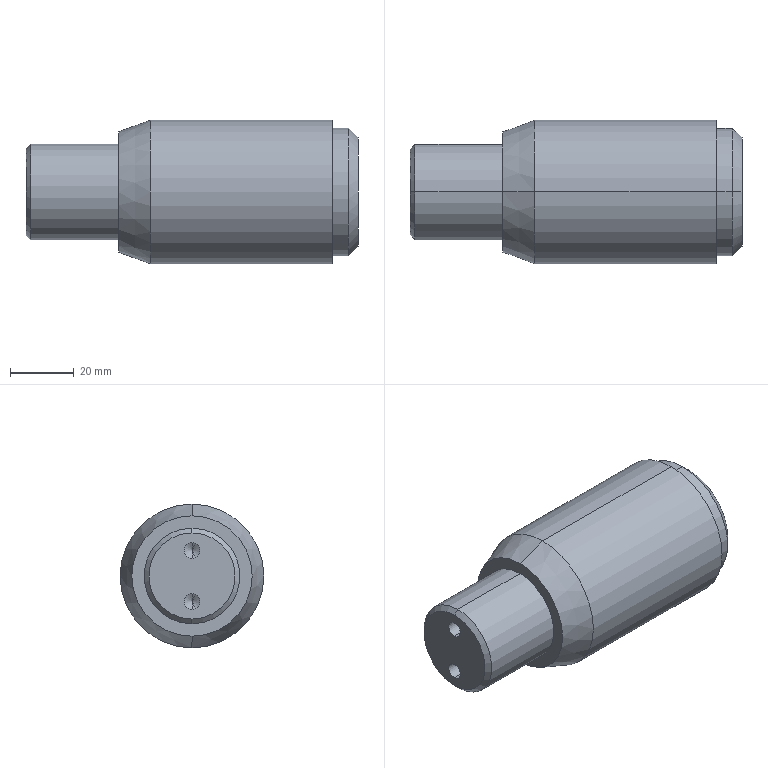Part | SolidWorks | features BaseBody 1 | 1 solid | 24 faces | box 104 x 45 x 45 mm | volume 133428 mm3 | cone 10 | cylinder 10 | plane 4 | commonest cylinder face diameters 5 x4 30 x2 40 x2 45 x2
STEP:
#1=CARTESIAN_POINT('',(-75.,0.,18.86));
#2=VERTEX_POINT('',#1);
#3=CARTESIAN_POINT('',(-75.,0.,-18.86));
#4=VERTEX_POINT('',#3);
#5=CARTESIAN_POINT('',(-75.,0.,0.));
#6=DIRECTION('',(-1.,0.,0.));
#7=DIRECTION('',(0.,0.,-1.));
#8=AXIS2_PLACEMENT_3D('',#5,#6,#7);
#9=CIRCLE('',#8,18.86);
#10=EDGE_CURVE('',#2,#4,#9,.T.);
#11=ORIENTED_EDGE('',*,*,#10,.F.);
#12=CARTESIAN_POINT('',(-65.,0.,22.5));
#13=VERTEX_POINT('',#12);
#14=CARTESIAN_POINT('',(-75.,0.,18.86));
#15=DIRECTION('',(0.9397,0.,0.342));
#16=VECTOR('',#15,1000.);
#17=LINE('',#14,#16);
#18=EDGE_CURVE('',#2,#13,#17,.T.);
#19=ORIENTED_EDGE('',*,*,#18,.T.);
#20=CARTESIAN_POINT('',(-65.,0.,-22.5));
#21=VERTEX_POINT('',#20);
#22=CARTESIAN_POINT('',(-65.,0.,0.));
#23=DIRECTION('',(1.,0.,0.));
#24=DIRECTION('',(0.,0.,-1.));
#25=AXIS2_PLACEMENT_3D('',#22,#23,#24);
#26=CIRCLE('',#25,22.5);
#27=EDGE_CURVE('',#21,#13,#26,.T.);
#28=ORIENTED_EDGE('',*,*,#27,.F.);
#29=CARTESIAN_POINT('',(-75.,0.,-18.86));
#30=DIRECTION('',(0.9397,0.,-0.342));
#31=VECTOR('',#30,1000.);
#32=LINE('',#29,#31);
#33=EDGE_CURVE('',#4,#21,#32,.T.);
#34=ORIENTED_EDGE('',*,*,#33,.F.);
#35=EDGE_LOOP('',(#11,#19,#28,#34));
#36=FACE_OUTER_BOUND('',#35,.T.);
#37=CARTESIAN_POINT('',(-75.,0.,0.));
#38=DIRECTION('',(1.,0.,0.));
#39=DIRECTION('',(0.,0.,-1.));
#40=AXIS2_PLACEMENT_3D('',#37,#38,#39);
#41=CONICAL_SURFACE('',#40,18.86,0.3491);
#42=ADVANCED_FACE('',(#36),#41,.T.);
#43=CARTESIAN_POINT('',(-89.,0.,-10.5));
#44=VERTEX_POINT('',#43);
#45=CARTESIAN_POINT('',(-89.,0.,-5.5));
#46=VERTEX_POINT('',#45);
#47=CARTESIAN_POINT('',(-89.,0.,-8.));
#48=DIRECTION('',(-1.,0.,0.));
#49=DIRECTION('',(0.,0.,1.));
#50=AXIS2_PLACEMENT_3D('',#47,#48,#49);
#51=CIRCLE('',#50,2.5);
#52=EDGE_CURVE('',#44,#46,#51,.T.);
#53=ORIENTED_EDGE('',*,*,#52,.F.);
#54=CARTESIAN_POINT('',(-104.,0.,-10.5));
#55=VERTEX_POINT('',#54);
#56=CARTESIAN_POINT('',(-104.,0.,-10.5));
#57=DIRECTION('',(-1.,0.,0.));
#58=VECTOR('',#57,1000.);
#59=LINE('',#56,#58);
#60=EDGE_CURVE('',#44,#55,#59,.T.);
#61=ORIENTED_EDGE('',*,*,#60,.T.);
#62=CARTESIAN_POINT('',(-104.,0.,-5.5));
#63=VERTEX_POINT('',#62);
#64=CARTESIAN_POINT('',(-104.,0.,-8.));
#65=DIRECTION('',(-1.,0.,0.));
#66=DIRECTION('',(0.,0.,1.));
#67=AXIS2_PLACEMENT_3D('',#64,#65,#66);
#68=CIRCLE('',#67,2.5);
#69=EDGE_CURVE('',#55,#63,#68,.T.);
#70=ORIENTED_EDGE('',*,*,#69,.T.);
#71=CARTESIAN_POINT('',(-104.,0.,-5.5));
#72=DIRECTION('',(-1.,0.,0.));
#73=VECTOR('',#72,1000.);
#74=LINE('',#71,#73);
#75=EDGE_CURVE('',#46,#63,#74,.T.);
#76=ORIENTED_EDGE('',*,*,#75,.F.);
#77=EDGE_LOOP('',(#53,#61,#70,#76));
#78=FACE_OUTER_BOUND('',#77,.T.);
#79=CARTESIAN_POINT('',(-104.,0.,-8.));
#80=DIRECTION('',(-1.,0.,0.));
#81=DIRECTION('',(0.,0.,1.));
#82=AXIS2_PLACEMENT_3D('',#79,#80,#81);
#83=CYLINDRICAL_SURFACE('',#82,2.5);
#84=ADVANCED_FACE('',(#78),#83,.F.);
#85=CARTESIAN_POINT('',(-87.498,0.,-8.));
#86=VERTEX_POINT('',#85);
#87=CARTESIAN_POINT('',(-89.,0.,-5.5));
#88=DIRECTION('',(-0.515,0.,0.8572));
#89=VECTOR('',#88,1000.);
#90=LINE('',#87,#89);
#91=EDGE_CURVE('',#86,#46,#90,.T.);
#92=ORIENTED_EDGE('',*,*,#91,.F.);
#93=CARTESIAN_POINT('',(-89.,0.,-10.5));
#94=DIRECTION('',(-0.515,0.,-0.8572));
#95=VECTOR('',#94,1000.);
#96=LINE('',#93,#95);
#97=EDGE_CURVE('',#86,#44,#96,.T.);
#98=ORIENTED_EDGE('',*,*,#97,.T.);
#99=ORIENTED_EDGE('',*,*,#52,.T.);
#100=EDGE_LOOP('',(#92,#98,#99));
#101=FACE_OUTER_BOUND('',#100,.T.);
#102=CARTESIAN_POINT('',(-89.,0.,-8.));
#103=DIRECTION('',(-1.,0.,0.));
#104=DIRECTION('',(0.,0.,1.));
#105=AXIS2_PLACEMENT_3D('',#102,#103,#104);
#106=CONICAL_SURFACE('',#105,2.5,1.03);
#107=ADVANCED_FACE('',(#101),#106,.F.);
#108=CARTESIAN_POINT('',(-89.,0.,5.5));
#109=VERTEX_POINT('',#108);
#110=CARTESIAN_POINT('',(-89.,0.,10.5));
#111=VERTEX_POINT('',#110);
#112=CARTESIAN_POINT('',(-89.,0.,8.));
#113=DIRECTION('',(-1.,0.,0.));
#114=DIRECTION('',(0.,0.,1.));
#115=AXIS2_PLACEMENT_3D('',#112,#113,#114);
#116=CIRCLE('',#115,2.5);
#117=EDGE_CURVE('',#109,#111,#116,.T.);
#118=ORIENTED_EDGE('',*,*,#117,.F.);
#119=CARTESIAN_POINT('',(-104.,0.,5.5));
#120=VERTEX_POINT('',#119);
#121=CARTESIAN_POINT('',(-104.,0.,5.5));
#122=DIRECTION('',(-1.,0.,0.));
#123=VECTOR('',#122,1000.);
#124=LINE('',#121,#123);
#125=EDGE_CURVE('',#109,#120,#124,.T.);
#126=ORIENTED_EDGE('',*,*,#125,.T.);
#127=CARTESIAN_POINT('',(-104.,0.,10.5));
#128=VERTEX_POINT('',#127);
#129=CARTESIAN_POINT('',(-104.,0.,8.));
#130=DIRECTION('',(-1.,0.,0.));
#131=DIRECTION('',(0.,0.,1.));
#132=AXIS2_PLACEMENT_3D('',#129,#130,#131);
#133=CIRCLE('',#132,2.5);
#134=EDGE_CURVE('',#120,#128,#133,.T.);
#135=ORIENTED_EDGE('',*,*,#134,.T.);
#136=CARTESIAN_POINT('',(-104.,0.,10.5));
#137=DIRECTION('',(-1.,0.,0.));
#138=VECTOR('',#137,1000.);
#139=LINE('',#136,#138);
#140=EDGE_CURVE('',#111,#128,#139,.T.);
#141=ORIENTED_EDGE('',*,*,#140,.F.);
#142=EDGE_LOOP('',(#118,#126,#135,#141));
#143=FACE_OUTER_BOUND('',#142,.T.);
#144=CARTESIAN_POINT('',(-104.,0.,8.));
#145=DIRECTION('',(-1.,0.,0.));
#146=DIRECTION('',(0.,0.,1.));
#147=AXIS2_PLACEMENT_3D('',#144,#145,#146);
#148=CYLINDRICAL_SURFACE('',#147,2.5);
#149=ADVANCED_FACE('',(#143),#148,.F.);
#150=CARTESIAN_POINT('',(-87.498,0.,8.));
#151=VERTEX_POINT('',#150);
#152=CARTESIAN_POINT('',(-89.,0.,10.5));
#153=DIRECTION('',(-0.515,0.,0.8572));
#154=VECTOR('',#153,1000.);
#155=LINE('',#152,#154);
#156=EDGE_CURVE('',#151,#111,#155,.T.);
#157=ORIENTED_EDGE('',*,*,#156,.F.);
#158=CARTESIAN_POINT('',(-89.,0.,5.5));
#159=DIRECTION('',(-0.515,0.,-0.8572));
#160=VECTOR('',#159,1000.);
#161=LINE('',#158,#160);
#162=EDGE_CURVE('',#151,#109,#161,.T.);
#163=ORIENTED_EDGE('',*,*,#162,.T.);
#164=ORIENTED_EDGE('',*,*,#117,.T.);
#165=EDGE_LOOP('',(#157,#163,#164));
#166=FACE_OUTER_BOUND('',#165,.T.);
#167=CARTESIAN_POINT('',(-89.,0.,8.));
#168=DIRECTION('',(-1.,0.,0.));
#169=DIRECTION('',(0.,0.,1.));
#170=AXIS2_PLACEMENT_3D('',#167,#168,#169);
#171=CONICAL_SURFACE('',#170,2.5,1.03);
#172=ADVANCED_FACE('',(#166),#171,.F.);
#173=CARTESIAN_POINT('',(-104.,0.,13.5));
#174=VERTEX_POINT('',#173);
#175=CARTESIAN_POINT('',(-104.,0.,-13.5));
#176=VERTEX_POINT('',#175);
#177=CARTESIAN_POINT('',(-104.,0.,0.));
#178=DIRECTION('',(-1.,0.,0.));
#179=DIRECTION('',(0.,0.,-1.));
#180=AXIS2_PLACEMENT_3D('',#177,#178,#179);
#181=CIRCLE('',#180,13.5);
#182=EDGE_CURVE('',#174,#176,#181,.T.);
#183=ORIENTED_EDGE('',*,*,#182,.F.);
#184=CARTESIAN_POINT('',(-102.5,0.,15.));
#185=VERTEX_POINT('',#184);
#186=CARTESIAN_POINT('',(-104.,0.,13.5));
#187=DIRECTION('',(0.7071,0.,0.7071));
#188=VECTOR('',#187,1000.);
#189=LINE('',#186,#188);
#190=EDGE_CURVE('',#174,#185,#189,.T.);
#191=ORIENTED_EDGE('',*,*,#190,.T.);
#192=CARTESIAN_POINT('',(-102.5,0.,-15.));
#193=VERTEX_POINT('',#192);
#194=CARTESIAN_POINT('',(-102.5,0.,0.));
#195=DIRECTION('',(1.,0.,0.));
#196=DIRECTION('',(0.,0.,-1.));
#197=AXIS2_PLACEMENT_3D('',#194,#195,#196);
#198=CIRCLE('',#197,15.);
#199=EDGE_CURVE('',#193,#185,#198,.T.);
#200=ORIENTED_EDGE('',*,*,#199,.F.);
#201=CARTESIAN_POINT('',(-104.,0.,-13.5));
#202=DIRECTION('',(0.7071,0.,-0.7071));
#203=VECTOR('',#202,1000.);
#204=LINE('',#201,#203);
#205=EDGE_CURVE('',#176,#193,#204,.T.);
#206=ORIENTED_EDGE('',*,*,#205,.F.);
#207=EDGE_LOOP('',(#183,#191,#200,#206));
#208=FACE_OUTER_BOUND('',#207,.T.);
#209=CARTESIAN_POINT('',(-104.,0.,0.));
#210=DIRECTION('',(1.,0.,0.));
#211=DIRECTION('',(0.,0.,-1.));
#212=AXIS2_PLACEMENT_3D('',#209,#210,#211);
#213=CONICAL_SURFACE('',#212,13.5,0.7854);
#214=ADVANCED_FACE('',(#208),#213,.T.);
#215=CARTESIAN_POINT('',(0.,0.,-17.));
#216=VERTEX_POINT('',#215);
#217=CARTESIAN_POINT('',(0.,0.,17.));
#218=VERTEX_POINT('',#217);
#219=CARTESIAN_POINT('',(0.,0.,0.));
#220=DIRECTION('',(1.,0.,0.));
#221=DIRECTION('',(0.,0.,1.));
#222=AXIS2_PLACEMENT_3D('',#219,#220,#221);
#223=CIRCLE('',#222,17.);
#224=EDGE_CURVE('',#216,#218,#223,.T.);
#225=ORIENTED_EDGE('',*,*,#224,.F.);
#226=CARTESIAN_POINT('',(-3.,0.,-20.));
#227=VERTEX_POINT('',#226);
#228=CARTESIAN_POINT('',(-3.,0.,-20.));
#229=DIRECTION('',(-0.7071,0.,-0.7071));
#230=VECTOR('',#229,1000.);
#231=LINE('',#228,#230);
#232=EDGE_CURVE('',#216,#227,#231,.T.);
#233=ORIENTED_EDGE('',*,*,#232,.T.);
#234=CARTESIAN_POINT('',(-3.,0.,20.));
#235=VERTEX_POINT('',#234);
#236=CARTESIAN_POINT('',(-3.,0.,0.));
#237=DIRECTION('',(-1.,0.,0.));
#238=DIRECTION('',(0.,0.,1.));
#239=AXIS2_PLACEMENT_3D('',#236,#237,#238);
#240=CIRCLE('',#239,20.);
#241=EDGE_CURVE('',#235,#227,#240,.T.);
#242=ORIENTED_EDGE('',*,*,#241,.F.);
#243=CARTESIAN_POINT('',(-3.,0.,20.));
#244=DIRECTION('',(-0.7071,0.,0.7071));
#245=VECTOR('',#244,1000.);
#246=LINE('',#243,#245);
#247=EDGE_CURVE('',#218,#235,#246,.T.);
#248=ORIENTED_EDGE('',*,*,#247,.F.);
#249=EDGE_LOOP('',(#225,#233,#242,#248));
#250=FACE_OUTER_BOUND('',#249,.T.);
#251=CARTESIAN_POINT('',(-3.,0.,0.));
#252=DIRECTION('',(-1.,0.,0.));
#253=DIRECTION('',(0.,0.,1.));
#254=AXIS2_PLACEMENT_3D('',#251,#252,#253);
#255=CONICAL_SURFACE('',#254,20.,0.7854);
#256=ADVANCED_FACE('',(#250),#255,.T.);
#257=CARTESIAN_POINT('',(-75.,0.,15.));
#258=VERTEX_POINT('',#257);
#259=CARTESIAN_POINT('',(-75.,0.,-15.));
#260=VERTEX_POINT('',#259);
#261=CARTESIAN_POINT('',(-75.,0.,0.));
#262=DIRECTION('',(-1.,0.,0.));
#263=DIRECTION('',(0.,0.,1.));
#264=AXIS2_PLACEMENT_3D('',#261,#262,#263);
#265=CIRCLE('',#264,15.);
#266=EDGE_CURVE('',#258,#260,#265,.T.);
#267=ORIENTED_EDGE('',*,*,#266,.T.);
#268=CARTESIAN_POINT('',(-104.,0.,-15.));
#269=DIRECTION('',(-1.,0.,0.));
#270=VECTOR('',#269,1000.);
#271=LINE('',#268,#270);
#272=EDGE_CURVE('',#260,#193,#271,.T.);
#273=ORIENTED_EDGE('',*,*,#272,.T.);
#274=ORIENTED_EDGE('',*,*,#199,.T.);
#275=CARTESIAN_POINT('',(-104.,0.,15.));
#276=DIRECTION('',(-1.,0.,0.));
#277=VECTOR('',#276,1000.);
#278=LINE('',#275,#277);
#279=EDGE_CURVE('',#258,#185,#278,.T.);
#280=ORIENTED_EDGE('',*,*,#279,.F.);
#281=EDGE_LOOP('',(#267,#273,#274,#280));
#282=FACE_OUTER_BOUND('',#281,.T.);
#283=CARTESIAN_POINT('',(-104.,0.,0.));
#284=DIRECTION('',(-1.,0.,0.));
#285=DIRECTION('',(0.,0.,1.));
#286=AXIS2_PLACEMENT_3D('',#283,#284,#285);
#287=CYLINDRICAL_SURFACE('',#286,15.);
#288=ADVANCED_FACE('',(#282),#287,.T.);
#289=CARTESIAN_POINT('',(-8.,0.,22.5));
#290=VERTEX_POINT('',#289);
#291=CARTESIAN_POINT('',(-8.,0.,-22.5));
#292=VERTEX_POINT('',#291);
#293=CARTESIAN_POINT('',(-8.,0.,0.));
#294=DIRECTION('',(-1.,0.,0.));
#295=DIRECTION('',(0.,0.,1.));
#296=AXIS2_PLACEMENT_3D('',#293,#294,#295);
#297=CIRCLE('',#296,22.5);
#298=EDGE_CURVE('',#290,#292,#297,.T.);
#299=ORIENTED_EDGE('',*,*,#298,.T.);
#300=CARTESIAN_POINT('',(-104.,0.,-22.5));
#301=DIRECTION('',(-1.,0.,0.));
#302=VECTOR('',#301,1000.);
#303=LINE('',#300,#302);
#304=EDGE_CURVE('',#292,#21,#303,.T.);
#305=ORIENTED_EDGE('',*,*,#304,.T.);
#306=ORIENTED_EDGE('',*,*,#27,.T.);
#307=CARTESIAN_POINT('',(-104.,0.,22.5));
#308=DIRECTION('',(-1.,0.,0.));
#309=VECTOR('',#308,1000.);
#310=LINE('',#307,#309);
#311=EDGE_CURVE('',#290,#13,#310,.T.);
#312=ORIENTED_EDGE('',*,*,#311,.F.);
#313=EDGE_LOOP('',(#299,#305,#306,#312));
#314=FACE_OUTER_BOUND('',#313,.T.);
#315=CARTESIAN_POINT('',(-104.,0.,0.));
#316=DIRECTION('',(-1.,0.,0.));
#317=DIRECTION('',(0.,0.,1.));
#318=AXIS2_PLACEMENT_3D('',#315,#316,#317);
#319=CYLINDRICAL_SURFACE('',#318,22.5);
#320=ADVANCED_FACE('',(#314),#319,.T.);
#321=ORIENTED_EDGE('',*,*,#241,.T.);
#322=CARTESIAN_POINT('',(-8.,0.,-20.));
#323=VERTEX_POINT('',#322);
#324=CARTESIAN_POINT('',(-104.,0.,-20.));
#325=DIRECTION('',(-1.,0.,0.));
#326=VECTOR('',#325,1000.);
#327=LINE('',#324,#326);
#328=EDGE_CURVE('',#227,#323,#327,.T.);
#329=ORIENTED_EDGE('',*,*,#328,.T.);
#330=CARTESIAN_POINT('',(-8.,0.,20.));
#331=VERTEX_POINT('',#330);
#332=CARTESIAN_POINT('',(-8.,0.,0.));
#333=DIRECTION('',(-1.,0.,0.));
#334=DIRECTION('',(0.,0.,1.));
#335=AXIS2_PLACEMENT_3D('',#332,#333,#334);
#336=CIRCLE('',#335,20.);
#337=EDGE_CURVE('',#331,#323,#336,.T.);
#338=ORIENTED_EDGE('',*,*,#337,.F.);
#339=CARTESIAN_POINT('',(-104.,0.,20.));
#340=DIRECTION('',(-1.,0.,0.));
#341=VECTOR('',#340,1000.);
#342=LINE('',#339,#341);
#343=EDGE_CURVE('',#235,#331,#342,.T.);
#344=ORIENTED_EDGE('',*,*,#343,.F.);
#345=EDGE_LOOP('',(#321,#329,#338,#344));
#346=FACE_OUTER_BOUND('',#345,.T.);
#347=CARTESIAN_POINT('',(-104.,0.,0.));
#348=DIRECTION('',(-1.,0.,0.));
#349=DIRECTION('',(0.,0.,1.));
#350=AXIS2_PLACEMENT_3D('',#347,#348,#349);
#351=CYLINDRICAL_SURFACE('',#350,20.);
#352=ADVANCED_FACE('',(#346),#351,.T.);
#353=CARTESIAN_POINT('',(-104.,0.,8.));
#354=DIRECTION('',(-1.,0.,0.));
#355=DIRECTION('',(0.,0.,1.));
#356=AXIS2_PLACEMENT_3D('',#353,#354,#355);
#357=CIRCLE('',#356,2.5);
#358=EDGE_CURVE('',#128,#120,#357,.T.);
#359=ORIENTED_EDGE('',*,*,#358,.F.);
#360=ORIENTED_EDGE('',*,*,#134,.F.);
#361=EDGE_LOOP('',(#359,#360));
#362=FACE_BOUND('',#361,.T.);
#363=CARTESIAN_POINT('',(-104.,0.,-8.));
#364=DIRECTION('',(-1.,0.,0.));
#365=DIRECTION('',(0.,0.,1.));
#366=AXIS2_PLACEMENT_3D('',#363,#364,#365);
#367=CIRCLE('',#366,2.5);
#368=EDGE_CURVE('',#63,#55,#367,.T.);
#369=ORIENTED_EDGE('',*,*,#368,.F.);
#370=ORIENTED_EDGE('',*,*,#69,.F.);
#371=EDGE_LOOP('',(#369,#370));
#372=FACE_BOUND('',#371,.T.);
#373=CARTESIAN_POINT('',(-104.,0.,0.));
#374=DIRECTION('',(-1.,0.,0.));
#375=DIRECTION('',(0.,0.,-1.));
#376=AXIS2_PLACEMENT_3D('',#373,#374,#375);
#377=CIRCLE('',#376,13.5);
#378=EDGE_CURVE('',#176,#174,#377,.T.);
#379=ORIENTED_EDGE('',*,*,#378,.T.);
#380=ORIENTED_EDGE('',*,*,#182,.T.);
#381=EDGE_LOOP('',(#379,#380));
#382=FACE_OUTER_BOUND('',#381,.T.);
#383=CARTESIAN_POINT('',(-104.,15.,0.));
#384=DIRECTION('',(1.,0.,0.));
#385=DIRECTION('',(0.,-1.,0.));
#386=AXIS2_PLACEMENT_3D('',#383,#384,#385);
#387=PLANE('',#386);
#388=ADVANCED_FACE('',(#362,#372,#382),#387,.F.);
#389=ORIENTED_EDGE('',*,*,#266,.F.);
#390=CARTESIAN_POINT('',(-75.,0.,0.));
#391=DIRECTION('',(-1.,0.,0.));
#392=DIRECTION('',(0.,0.,1.));
#393=AXIS2_PLACEMENT_3D('',#390,#391,#392);
#394=CIRCLE('',#393,15.);
#395=EDGE_CURVE('',#260,#258,#394,.T.);
#396=ORIENTED_EDGE('',*,*,#395,.F.);
#397=EDGE_LOOP('',(#389,#396));
#398=FACE_BOUND('',#397,.T.);
#399=CARTESIAN_POINT('',(-75.,0.,0.));
#400=DIRECTION('',(-1.,0.,0.));
#401=DIRECTION('',(0.,0.,-1.));
#402=AXIS2_PLACEMENT_3D('',#399,#400,#401);
#403=CIRCLE('',#402,18.86);
#404=EDGE_CURVE('',#4,#2,#403,.T.);
#405=ORIENTED_EDGE('',*,*,#404,.T.);
#406=ORIENTED_EDGE('',*,*,#10,.T.);
#407=EDGE_LOOP('',(#405,#406));
#408=FACE_OUTER_BOUND('',#407,.T.);
#409=CARTESIAN_POINT('',(-75.,22.5,0.));
#410=DIRECTION('',(1.,0.,0.));
#411=DIRECTION('',(0.,-1.,0.));
#412=AXIS2_PLACEMENT_3D('',#409,#410,#411);
#413=PLANE('',#412);
#414=ADVANCED_FACE('',(#398,#408),#413,.F.);
#415=ORIENTED_EDGE('',*,*,#337,.T.);
#416=CARTESIAN_POINT('',(-8.,0.,0.));
#417=DIRECTION('',(-1.,0.,0.));
#418=DIRECTION('',(0.,0.,1.));
#419=AXIS2_PLACEMENT_3D('',#416,#417,#418);
#420=CIRCLE('',#419,20.);
#421=EDGE_CURVE('',#323,#331,#420,.T.);
#422=ORIENTED_EDGE('',*,*,#421,.T.);
#423=EDGE_LOOP('',(#415,#422));
#424=FACE_BOUND('',#423,.T.);
#425=ORIENTED_EDGE('',*,*,#298,.F.);
#426=CARTESIAN_POINT('',(-8.,0.,0.));
#427=DIRECTION('',(-1.,0.,0.));
#428=DIRECTION('',(0.,0.,1.));
#429=AXIS2_PLACEMENT_3D('',#426,#427,#428);
#430=CIRCLE('',#429,22.5);
#431=EDGE_CURVE('',#292,#290,#430,.T.);
#432=ORIENTED_EDGE('',*,*,#431,.F.);
#433=EDGE_LOOP('',(#425,#432));
#434=FACE_OUTER_BOUND('',#433,.T.);
#435=CARTESIAN_POINT('',(-8.,20.,0.));
#436=DIRECTION('',(-1.,0.,0.));
#437=DIRECTION('',(0.,0.,1.));
#438=AXIS2_PLACEMENT_3D('',#435,#436,#437);
#439=PLANE('',#438);
#440=ADVANCED_FACE('',(#424,#434),#439,.F.);
#441=CARTESIAN_POINT('',(0.,0.,0.));
#442=DIRECTION('',(1.,0.,0.));
#443=DIRECTION('',(0.,0.,1.));
#444=AXIS2_PLACEMENT_3D('',#441,#442,#443);
#445=CIRCLE('',#444,17.);
#446=EDGE_CURVE('',#218,#216,#445,.T.);
#447=ORIENTED_EDGE('',*,*,#446,.T.);
#448=ORIENTED_EDGE('',*,*,#224,.T.);
#449=EDGE_LOOP('',(#447,#448));
#450=FACE_OUTER_BOUND('',#449,.T.);
#451=CARTESIAN_POINT('',(0.,0.,0.));
#452=DIRECTION('',(-1.,0.,0.));
#453=DIRECTION('',(0.,0.,1.));
#454=AXIS2_PLACEMENT_3D('',#451,#452,#453);
#455=PLANE('',#454);
#456=ADVANCED_FACE('',(#450),#455,.F.);
#457=ORIENTED_EDGE('',*,*,#328,.F.);
#458=CARTESIAN_POINT('',(-3.,0.,0.));
#459=DIRECTION('',(-1.,0.,0.));
#460=DIRECTION('',(0.,0.,1.));
#461=AXIS2_PLACEMENT_3D('',#458,#459,#460);
#462=CIRCLE('',#461,20.);
#463=EDGE_CURVE('',#227,#235,#462,.T.);
#464=ORIENTED_EDGE('',*,*,#463,.T.);
#465=ORIENTED_EDGE('',*,*,#343,.T.);
#466=ORIENTED_EDGE('',*,*,#421,.F.);
#467=EDGE_LOOP('',(#457,#464,#465,#466));
#468=FACE_OUTER_BOUND('',#467,.T.);
#469=CARTESIAN_POINT('',(-104.,0.,0.));
#470=DIRECTION('',(-1.,0.,0.));
#471=DIRECTION('',(0.,0.,1.));
#472=AXIS2_PLACEMENT_3D('',#469,#470,#471);
#473=CYLINDRICAL_SURFACE('',#472,20.);
#474=ADVANCED_FACE('',(#468),#473,.T.);
#475=ORIENTED_EDGE('',*,*,#304,.F.);
#476=ORIENTED_EDGE('',*,*,#431,.T.);
#477=ORIENTED_EDGE('',*,*,#311,.T.);
#478=CARTESIAN_POINT('',(-65.,0.,0.));
#479=DIRECTION('',(1.,0.,0.));
#480=DIRECTION('',(0.,0.,-1.));
#481=AXIS2_PLACEMENT_3D('',#478,#479,#480);
#482=CIRCLE('',#481,22.5);
#483=EDGE_CURVE('',#13,#21,#482,.T.);
#484=ORIENTED_EDGE('',*,*,#483,.T.);
#485=EDGE_LOOP('',(#475,#476,#477,#484));
#486=FACE_OUTER_BOUND('',#485,.T.);
#487=CARTESIAN_POINT('',(-104.,0.,0.));
#488=DIRECTION('',(-1.,0.,0.));
#489=DIRECTION('',(0.,0.,1.));
#490=AXIS2_PLACEMENT_3D('',#487,#488,#489);
#491=CYLINDRICAL_SURFACE('',#490,22.5);
#492=ADVANCED_FACE('',(#486),#491,.T.);
#493=ORIENTED_EDGE('',*,*,#272,.F.);
#494=ORIENTED_EDGE('',*,*,#395,.T.);
#495=ORIENTED_EDGE('',*,*,#279,.T.);
#496=CARTESIAN_POINT('',(-102.5,0.,0.));
#497=DIRECTION('',(1.,0.,0.));
#498=DIRECTION('',(0.,0.,-1.));
#499=AXIS2_PLACEMENT_3D('',#496,#497,#498);
#500=CIRCLE('',#499,15.);
#501=EDGE_CURVE('',#185,#193,#500,.T.);
#502=ORIENTED_EDGE('',*,*,#501,.T.);
#503=EDGE_LOOP('',(#493,#494,#495,#502));
#504=FACE_OUTER_BOUND('',#503,.T.);
#505=CARTESIAN_POINT('',(-104.,0.,0.));
#506=DIRECTION('',(-1.,0.,0.));
#507=DIRECTION('',(0.,0.,1.));
#508=AXIS2_PLACEMENT_3D('',#505,#506,#507);
#509=CYLINDRICAL_SURFACE('',#508,15.);
#510=ADVANCED_FACE('',(#504),#509,.T.);
#511=ORIENTED_EDGE('',*,*,#232,.F.);
#512=ORIENTED_EDGE('',*,*,#446,.F.);
#513=ORIENTED_EDGE('',*,*,#247,.T.);
#514=ORIENTED_EDGE('',*,*,#463,.F.);
#515=EDGE_LOOP('',(#511,#512,#513,#514));
#516=FACE_OUTER_BOUND('',#515,.T.);
#517=CARTESIAN_POINT('',(-3.,0.,0.));
#518=DIRECTION('',(-1.,0.,0.));
#519=DIRECTION('',(0.,0.,1.));
#520=AXIS2_PLACEMENT_3D('',#517,#518,#519);
#521=CONICAL_SURFACE('',#520,20.,0.7854);
#522=ADVANCED_FACE('',(#516),#521,.T.);
#523=ORIENTED_EDGE('',*,*,#190,.F.);
#524=ORIENTED_EDGE('',*,*,#378,.F.);
#525=ORIENTED_EDGE('',*,*,#205,.T.);
#526=ORIENTED_EDGE('',*,*,#501,.F.);
#527=EDGE_LOOP('',(#523,#524,#525,#526));
#528=FACE_OUTER_BOUND('',#527,.T.);
#529=CARTESIAN_POINT('',(-104.,0.,0.));
#530=DIRECTION('',(1.,0.,0.));
#531=DIRECTION('',(0.,0.,-1.));
#532=AXIS2_PLACEMENT_3D('',#529,#530,#531);
#533=CONICAL_SURFACE('',#532,13.5,0.7854);
#534=ADVANCED_FACE('',(#528),#533,.T.);
#535=ORIENTED_EDGE('',*,*,#162,.F.);
#536=ORIENTED_EDGE('',*,*,#156,.T.);
#537=CARTESIAN_POINT('',(-89.,0.,8.));
#538=DIRECTION('',(-1.,0.,0.));
#539=DIRECTION('',(0.,0.,1.));
#540=AXIS2_PLACEMENT_3D('',#537,#538,#539);
#541=CIRCLE('',#540,2.5);
#542=EDGE_CURVE('',#111,#109,#541,.T.);
#543=ORIENTED_EDGE('',*,*,#542,.T.);
#544=EDGE_LOOP('',(#535,#536,#543));
#545=FACE_OUTER_BOUND('',#544,.T.);
#546=CARTESIAN_POINT('',(-89.,0.,8.));
#547=DIRECTION('',(-1.,0.,0.));
#548=DIRECTION('',(0.,0.,1.));
#549=AXIS2_PLACEMENT_3D('',#546,#547,#548);
#550=CONICAL_SURFACE('',#549,2.5,1.03);
#551=ADVANCED_FACE('',(#545),#550,.F.);
#552=ORIENTED_EDGE('',*,*,#125,.F.);
#553=ORIENTED_EDGE('',*,*,#542,.F.);
#554=ORIENTED_EDGE('',*,*,#140,.T.);
#555=ORIENTED_EDGE('',*,*,#358,.T.);
#556=EDGE_LOOP('',(#552,#553,#554,#555));
#557=FACE_OUTER_BOUND('',#556,.T.);
#558=CARTESIAN_POINT('',(-104.,0.,8.));
#559=DIRECTION('',(-1.,0.,0.));
#560=DIRECTION('',(0.,0.,1.));
#561=AXIS2_PLACEMENT_3D('',#558,#559,#560);
#562=CYLINDRICAL_SURFACE('',#561,2.5);
#563=ADVANCED_FACE('',(#557),#562,.F.);
#564=ORIENTED_EDGE('',*,*,#97,.F.);
#565=ORIENTED_EDGE('',*,*,#91,.T.);
#566=CARTESIAN_POINT('',(-89.,0.,-8.));
#567=DIRECTION('',(-1.,0.,0.));
#568=DIRECTION('',(0.,0.,1.));
#569=AXIS2_PLACEMENT_3D('',#566,#567,#568);
#570=CIRCLE('',#569,2.5);
#571=EDGE_CURVE('',#46,#44,#570,.T.);
#572=ORIENTED_EDGE('',*,*,#571,.T.);
#573=EDGE_LOOP('',(#564,#565,#572));
#574=FACE_OUTER_BOUND('',#573,.T.);
#575=CARTESIAN_POINT('',(-89.,0.,-8.));
#576=DIRECTION('',(-1.,0.,0.));
#577=DIRECTION('',(0.,0.,1.));
#578=AXIS2_PLACEMENT_3D('',#575,#576,#577);
#579=CONICAL_SURFACE('',#578,2.5,1.03);
#580=ADVANCED_FACE('',(#574),#579,.F.);
#581=ORIENTED_EDGE('',*,*,#60,.F.);
#582=ORIENTED_EDGE('',*,*,#571,.F.);
#583=ORIENTED_EDGE('',*,*,#75,.T.);
#584=ORIENTED_EDGE('',*,*,#368,.T.);
#585=EDGE_LOOP('',(#581,#582,#583,#584));
#586=FACE_OUTER_BOUND('',#585,.T.);
#587=CARTESIAN_POINT('',(-104.,0.,-8.));
#588=DIRECTION('',(-1.,0.,0.));
#589=DIRECTION('',(0.,0.,1.));
#590=AXIS2_PLACEMENT_3D('',#587,#588,#589);
#591=CYLINDRICAL_SURFACE('',#590,2.5);
#592=ADVANCED_FACE('',(#586),#591,.F.);
#593=ORIENTED_EDGE('',*,*,#18,.F.);
#594=ORIENTED_EDGE('',*,*,#404,.F.);
#595=ORIENTED_EDGE('',*,*,#33,.T.);
#596=ORIENTED_EDGE('',*,*,#483,.F.);
#597=EDGE_LOOP('',(#593,#594,#595,#596));
#598=FACE_OUTER_BOUND('',#597,.T.);
#599=CARTESIAN_POINT('',(-75.,0.,0.));
#600=DIRECTION('',(1.,0.,0.));
#601=DIRECTION('',(0.,0.,-1.));
#602=AXIS2_PLACEMENT_3D('',#599,#600,#601);
#603=CONICAL_SURFACE('',#602,18.86,0.3491);
#604=ADVANCED_FACE('',(#598),#603,.T.);
#605=CLOSED_SHELL('',(#42,#84,#107,#149,#172,#214,#256,#288,#320,#352,#388,#414,#440,#456,#474,#492,#510,#522,#534,#551,#563,#580,#592,#604));
#606=MANIFOLD_SOLID_BREP('',#605);
#607=CARTESIAN_POINT('',(0.,0.,0.));
#608=DIRECTION('',(0.,0.,1.));
#609=DIRECTION('',(1.,0.,0.));
#610=AXIS2_PLACEMENT_3D('',#607,#608,#609);
#611=(LENGTH_UNIT()NAMED_UNIT(*)SI_UNIT(.MILLI.,.METRE.));
#612=UNCERTAINTY_MEASURE_WITH_UNIT(LENGTH_MEASURE(0.00001),#611,'','');
#613=(NAMED_UNIT(*)PLANE_ANGLE_UNIT()SI_UNIT($,.RADIAN.));
#614=(NAMED_UNIT(*)SI_UNIT($,.STERADIAN.)SOLID_ANGLE_UNIT());
#615=(GEOMETRIC_REPRESENTATION_CONTEXT(3)GLOBAL_UNCERTAINTY_ASSIGNED_CONTEXT((#612))GLOBAL_UNIT_ASSIGNED_CONTEXT((#611,#613,#614))REPRESENTATION_CONTEXT('',''));
#616=ADVANCED_BREP_SHAPE_REPRESENTATION('',(#606,#610),#615);